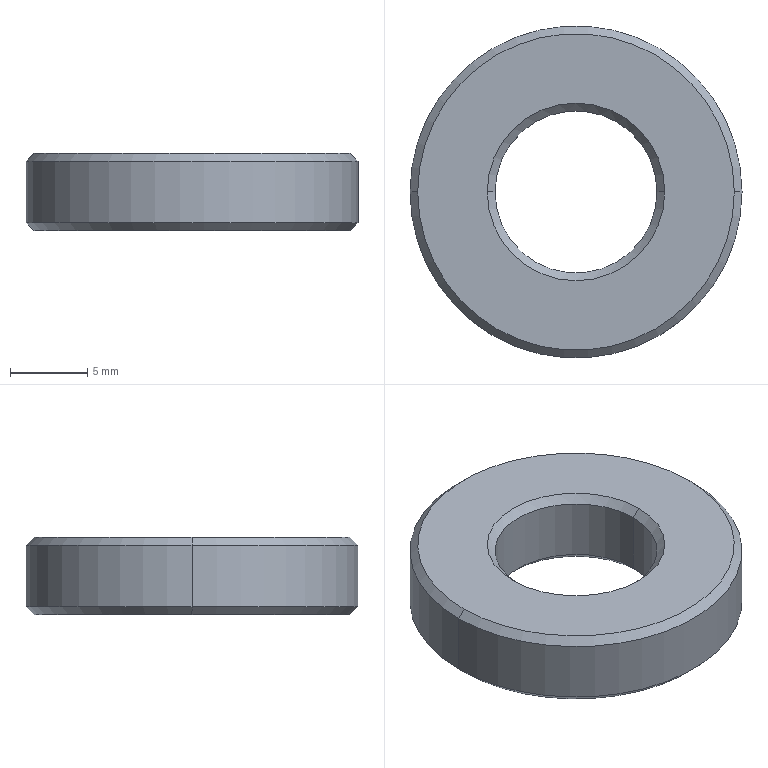Part | SolidWorks | features Chamfer 1, Extrusion 1 | 1 solid | 14 faces | box 21.5 x 21.5 x 5 mm | volume 1357 mm3 | cone 8 | cylinder 4 | plane 2 | commonest cylinder face diameters 10.5 x2 21.5 x2
STEP:
#1=CARTESIAN_POINT('',(10.25,0.,5.));
#2=VERTEX_POINT('',#1);
#3=CARTESIAN_POINT('',(-10.25,0.,5.));
#4=VERTEX_POINT('',#3);
#5=CARTESIAN_POINT('',(0.,0.,5.));
#6=DIRECTION('',(0.,0.,1.));
#7=DIRECTION('',(1.,0.,0.));
#8=AXIS2_PLACEMENT_3D('',#5,#6,#7);
#9=CIRCLE('',#8,10.25);
#10=EDGE_CURVE('',#2,#4,#9,.T.);
#11=ORIENTED_EDGE('',*,*,#10,.F.);
#12=CARTESIAN_POINT('',(10.75,0.,4.5));
#13=VERTEX_POINT('',#12);
#14=CARTESIAN_POINT('',(10.25,0.,5.));
#15=DIRECTION('',(0.7071,0.,-0.7071));
#16=VECTOR('',#15,1000.);
#17=LINE('',#14,#16);
#18=EDGE_CURVE('',#2,#13,#17,.T.);
#19=ORIENTED_EDGE('',*,*,#18,.T.);
#20=CARTESIAN_POINT('',(-10.75,0.,4.5));
#21=VERTEX_POINT('',#20);
#22=CARTESIAN_POINT('',(0.,0.,4.5));
#23=DIRECTION('',(0.,0.,-1.));
#24=DIRECTION('',(1.,0.,0.));
#25=AXIS2_PLACEMENT_3D('',#22,#23,#24);
#26=CIRCLE('',#25,10.75);
#27=EDGE_CURVE('',#21,#13,#26,.T.);
#28=ORIENTED_EDGE('',*,*,#27,.F.);
#29=CARTESIAN_POINT('',(-10.25,0.,5.));
#30=DIRECTION('',(-0.7071,0.,-0.7071));
#31=VECTOR('',#30,1000.);
#32=LINE('',#29,#31);
#33=EDGE_CURVE('',#4,#21,#32,.T.);
#34=ORIENTED_EDGE('',*,*,#33,.F.);
#35=EDGE_LOOP('',(#11,#19,#28,#34));
#36=FACE_OUTER_BOUND('',#35,.T.);
#37=CARTESIAN_POINT('',(0.,0.,5.));
#38=DIRECTION('',(0.,0.,-1.));
#39=DIRECTION('',(-1.,0.,0.));
#40=AXIS2_PLACEMENT_3D('',#37,#38,#39);
#41=CONICAL_SURFACE('',#40,10.25,0.7854);
#42=ADVANCED_FACE('',(#36),#41,.T.);
#43=CARTESIAN_POINT('',(-5.25,0.,4.5));
#44=VERTEX_POINT('',#43);
#45=CARTESIAN_POINT('',(5.25,0.,4.5));
#46=VERTEX_POINT('',#45);
#47=CARTESIAN_POINT('',(0.,0.,4.5));
#48=DIRECTION('',(0.,0.,1.));
#49=DIRECTION('',(1.,0.,0.));
#50=AXIS2_PLACEMENT_3D('',#47,#48,#49);
#51=CIRCLE('',#50,5.25);
#52=EDGE_CURVE('',#44,#46,#51,.T.);
#53=ORIENTED_EDGE('',*,*,#52,.F.);
#54=CARTESIAN_POINT('',(-5.75,0.,5.));
#55=VERTEX_POINT('',#54);
#56=CARTESIAN_POINT('',(-5.25,0.,4.5));
#57=DIRECTION('',(-0.7071,0.,0.7071));
#58=VECTOR('',#57,1000.);
#59=LINE('',#56,#58);
#60=EDGE_CURVE('',#44,#55,#59,.T.);
#61=ORIENTED_EDGE('',*,*,#60,.T.);
#62=CARTESIAN_POINT('',(5.75,0.,5.));
#63=VERTEX_POINT('',#62);
#64=CARTESIAN_POINT('',(0.,0.,5.));
#65=DIRECTION('',(0.,0.,-1.));
#66=DIRECTION('',(1.,0.,0.));
#67=AXIS2_PLACEMENT_3D('',#64,#65,#66);
#68=CIRCLE('',#67,5.75);
#69=EDGE_CURVE('',#63,#55,#68,.T.);
#70=ORIENTED_EDGE('',*,*,#69,.F.);
#71=CARTESIAN_POINT('',(5.25,0.,4.5));
#72=DIRECTION('',(0.7071,0.,0.7071));
#73=VECTOR('',#72,1000.);
#74=LINE('',#71,#73);
#75=EDGE_CURVE('',#46,#63,#74,.T.);
#76=ORIENTED_EDGE('',*,*,#75,.F.);
#77=EDGE_LOOP('',(#53,#61,#70,#76));
#78=FACE_OUTER_BOUND('',#77,.T.);
#79=CARTESIAN_POINT('',(0.,0.,4.5));
#80=DIRECTION('',(0.,0.,1.));
#81=DIRECTION('',(1.,0.,0.));
#82=AXIS2_PLACEMENT_3D('',#79,#80,#81);
#83=CONICAL_SURFACE('',#82,5.25,0.7854);
#84=ADVANCED_FACE('',(#78),#83,.F.);
#85=CARTESIAN_POINT('',(5.25,0.,0.5));
#86=VERTEX_POINT('',#85);
#87=CARTESIAN_POINT('',(-5.25,0.,0.5));
#88=VERTEX_POINT('',#87);
#89=CARTESIAN_POINT('',(0.,0.,0.5));
#90=DIRECTION('',(0.,0.,-1.));
#91=DIRECTION('',(1.,0.,0.));
#92=AXIS2_PLACEMENT_3D('',#89,#90,#91);
#93=CIRCLE('',#92,5.25);
#94=EDGE_CURVE('',#86,#88,#93,.T.);
#95=ORIENTED_EDGE('',*,*,#94,.F.);
#96=CARTESIAN_POINT('',(5.75,0.,0.));
#97=VERTEX_POINT('',#96);
#98=CARTESIAN_POINT('',(5.75,0.,0.));
#99=DIRECTION('',(0.7071,0.,-0.7071));
#100=VECTOR('',#99,1000.);
#101=LINE('',#98,#100);
#102=EDGE_CURVE('',#86,#97,#101,.T.);
#103=ORIENTED_EDGE('',*,*,#102,.T.);
#104=CARTESIAN_POINT('',(-5.75,0.,0.));
#105=VERTEX_POINT('',#104);
#106=CARTESIAN_POINT('',(0.,0.,0.));
#107=DIRECTION('',(0.,0.,1.));
#108=DIRECTION('',(1.,0.,0.));
#109=AXIS2_PLACEMENT_3D('',#106,#107,#108);
#110=CIRCLE('',#109,5.75);
#111=EDGE_CURVE('',#105,#97,#110,.T.);
#112=ORIENTED_EDGE('',*,*,#111,.F.);
#113=CARTESIAN_POINT('',(-5.75,0.,0.));
#114=DIRECTION('',(-0.7071,0.,-0.7071));
#115=VECTOR('',#114,1000.);
#116=LINE('',#113,#115);
#117=EDGE_CURVE('',#88,#105,#116,.T.);
#118=ORIENTED_EDGE('',*,*,#117,.F.);
#119=EDGE_LOOP('',(#95,#103,#112,#118));
#120=FACE_OUTER_BOUND('',#119,.T.);
#121=CARTESIAN_POINT('',(0.,0.,0.));
#122=DIRECTION('',(0.,0.,-1.));
#123=DIRECTION('',(-1.,0.,0.));
#124=AXIS2_PLACEMENT_3D('',#121,#122,#123);
#125=CONICAL_SURFACE('',#124,5.75,0.7854);
#126=ADVANCED_FACE('',(#120),#125,.F.);
#127=CARTESIAN_POINT('',(-10.25,0.,0.));
#128=VERTEX_POINT('',#127);
#129=CARTESIAN_POINT('',(10.25,0.,0.));
#130=VERTEX_POINT('',#129);
#131=CARTESIAN_POINT('',(0.,0.,0.));
#132=DIRECTION('',(0.,0.,-1.));
#133=DIRECTION('',(1.,0.,0.));
#134=AXIS2_PLACEMENT_3D('',#131,#132,#133);
#135=CIRCLE('',#134,10.25);
#136=EDGE_CURVE('',#128,#130,#135,.T.);
#137=ORIENTED_EDGE('',*,*,#136,.F.);
#138=CARTESIAN_POINT('',(-10.75,0.,0.5));
#139=VERTEX_POINT('',#138);
#140=CARTESIAN_POINT('',(-10.75,0.,0.5));
#141=DIRECTION('',(-0.7071,0.,0.7071));
#142=VECTOR('',#141,1000.);
#143=LINE('',#140,#142);
#144=EDGE_CURVE('',#128,#139,#143,.T.);
#145=ORIENTED_EDGE('',*,*,#144,.T.);
#146=CARTESIAN_POINT('',(10.75,0.,0.5));
#147=VERTEX_POINT('',#146);
#148=CARTESIAN_POINT('',(0.,0.,0.5));
#149=DIRECTION('',(0.,0.,1.));
#150=DIRECTION('',(1.,0.,0.));
#151=AXIS2_PLACEMENT_3D('',#148,#149,#150);
#152=CIRCLE('',#151,10.75);
#153=EDGE_CURVE('',#147,#139,#152,.T.);
#154=ORIENTED_EDGE('',*,*,#153,.F.);
#155=CARTESIAN_POINT('',(10.75,0.,0.5));
#156=DIRECTION('',(0.7071,0.,0.7071));
#157=VECTOR('',#156,1000.);
#158=LINE('',#155,#157);
#159=EDGE_CURVE('',#130,#147,#158,.T.);
#160=ORIENTED_EDGE('',*,*,#159,.F.);
#161=EDGE_LOOP('',(#137,#145,#154,#160));
#162=FACE_OUTER_BOUND('',#161,.T.);
#163=CARTESIAN_POINT('',(0.,0.,0.5));
#164=DIRECTION('',(0.,0.,1.));
#165=DIRECTION('',(1.,0.,0.));
#166=AXIS2_PLACEMENT_3D('',#163,#164,#165);
#167=CONICAL_SURFACE('',#166,10.75,0.7854);
#168=ADVANCED_FACE('',(#162),#167,.T.);
#169=ORIENTED_EDGE('',*,*,#52,.T.);
#170=CARTESIAN_POINT('',(5.25,0.,5.));
#171=DIRECTION('',(0.,0.,-1.));
#172=VECTOR('',#171,1000.);
#173=LINE('',#170,#172);
#174=EDGE_CURVE('',#46,#86,#173,.T.);
#175=ORIENTED_EDGE('',*,*,#174,.T.);
#176=ORIENTED_EDGE('',*,*,#94,.T.);
#177=CARTESIAN_POINT('',(-5.25,0.,5.));
#178=DIRECTION('',(0.,0.,-1.));
#179=VECTOR('',#178,1000.);
#180=LINE('',#177,#179);
#181=EDGE_CURVE('',#44,#88,#180,.T.);
#182=ORIENTED_EDGE('',*,*,#181,.F.);
#183=EDGE_LOOP('',(#169,#175,#176,#182));
#184=FACE_OUTER_BOUND('',#183,.T.);
#185=CARTESIAN_POINT('',(0.,0.,5.));
#186=DIRECTION('',(0.,0.,-1.));
#187=DIRECTION('',(-1.,0.,0.));
#188=AXIS2_PLACEMENT_3D('',#185,#186,#187);
#189=CYLINDRICAL_SURFACE('',#188,5.25);
#190=ADVANCED_FACE('',(#184),#189,.F.);
#191=ORIENTED_EDGE('',*,*,#27,.T.);
#192=CARTESIAN_POINT('',(10.75,0.,5.));
#193=DIRECTION('',(0.,0.,-1.));
#194=VECTOR('',#193,1000.);
#195=LINE('',#192,#194);
#196=EDGE_CURVE('',#13,#147,#195,.T.);
#197=ORIENTED_EDGE('',*,*,#196,.T.);
#198=ORIENTED_EDGE('',*,*,#153,.T.);
#199=CARTESIAN_POINT('',(-10.75,0.,5.));
#200=DIRECTION('',(0.,0.,-1.));
#201=VECTOR('',#200,1000.);
#202=LINE('',#199,#201);
#203=EDGE_CURVE('',#21,#139,#202,.T.);
#204=ORIENTED_EDGE('',*,*,#203,.F.);
#205=EDGE_LOOP('',(#191,#197,#198,#204));
#206=FACE_OUTER_BOUND('',#205,.T.);
#207=CARTESIAN_POINT('',(0.,0.,5.));
#208=DIRECTION('',(0.,0.,-1.));
#209=DIRECTION('',(-1.,0.,0.));
#210=AXIS2_PLACEMENT_3D('',#207,#208,#209);
#211=CYLINDRICAL_SURFACE('',#210,10.75);
#212=ADVANCED_FACE('',(#206),#211,.T.);
#213=ORIENTED_EDGE('',*,*,#69,.T.);
#214=CARTESIAN_POINT('',(0.,0.,5.));
#215=DIRECTION('',(0.,0.,-1.));
#216=DIRECTION('',(1.,0.,0.));
#217=AXIS2_PLACEMENT_3D('',#214,#215,#216);
#218=CIRCLE('',#217,5.75);
#219=EDGE_CURVE('',#55,#63,#218,.T.);
#220=ORIENTED_EDGE('',*,*,#219,.T.);
#221=EDGE_LOOP('',(#213,#220));
#222=FACE_BOUND('',#221,.T.);
#223=CARTESIAN_POINT('',(0.,0.,5.));
#224=DIRECTION('',(0.,0.,1.));
#225=DIRECTION('',(1.,0.,0.));
#226=AXIS2_PLACEMENT_3D('',#223,#224,#225);
#227=CIRCLE('',#226,10.25);
#228=EDGE_CURVE('',#4,#2,#227,.T.);
#229=ORIENTED_EDGE('',*,*,#228,.T.);
#230=ORIENTED_EDGE('',*,*,#10,.T.);
#231=EDGE_LOOP('',(#229,#230));
#232=FACE_OUTER_BOUND('',#231,.T.);
#233=CARTESIAN_POINT('',(0.,0.,5.));
#234=DIRECTION('',(0.,0.,1.));
#235=DIRECTION('',(1.,0.,0.));
#236=AXIS2_PLACEMENT_3D('',#233,#234,#235);
#237=PLANE('',#236);
#238=ADVANCED_FACE('',(#222,#232),#237,.T.);
#239=CARTESIAN_POINT('',(0.,0.,0.));
#240=DIRECTION('',(0.,0.,-1.));
#241=DIRECTION('',(1.,0.,0.));
#242=AXIS2_PLACEMENT_3D('',#239,#240,#241);
#243=CIRCLE('',#242,10.25);
#244=EDGE_CURVE('',#130,#128,#243,.T.);
#245=ORIENTED_EDGE('',*,*,#244,.T.);
#246=ORIENTED_EDGE('',*,*,#136,.T.);
#247=EDGE_LOOP('',(#245,#246));
#248=FACE_OUTER_BOUND('',#247,.T.);
#249=ORIENTED_EDGE('',*,*,#111,.T.);
#250=CARTESIAN_POINT('',(0.,0.,0.));
#251=DIRECTION('',(0.,0.,1.));
#252=DIRECTION('',(1.,0.,0.));
#253=AXIS2_PLACEMENT_3D('',#250,#251,#252);
#254=CIRCLE('',#253,5.75);
#255=EDGE_CURVE('',#97,#105,#254,.T.);
#256=ORIENTED_EDGE('',*,*,#255,.T.);
#257=EDGE_LOOP('',(#249,#256));
#258=FACE_BOUND('',#257,.T.);
#259=CARTESIAN_POINT('',(0.,0.,0.));
#260=DIRECTION('',(0.,0.,1.));
#261=DIRECTION('',(1.,0.,0.));
#262=AXIS2_PLACEMENT_3D('',#259,#260,#261);
#263=PLANE('',#262);
#264=ADVANCED_FACE('',(#248,#258),#263,.F.);
#265=ORIENTED_EDGE('',*,*,#196,.F.);
#266=CARTESIAN_POINT('',(0.,0.,4.5));
#267=DIRECTION('',(0.,0.,-1.));
#268=DIRECTION('',(1.,0.,0.));
#269=AXIS2_PLACEMENT_3D('',#266,#267,#268);
#270=CIRCLE('',#269,10.75);
#271=EDGE_CURVE('',#13,#21,#270,.T.);
#272=ORIENTED_EDGE('',*,*,#271,.T.);
#273=ORIENTED_EDGE('',*,*,#203,.T.);
#274=CARTESIAN_POINT('',(0.,0.,0.5));
#275=DIRECTION('',(0.,0.,1.));
#276=DIRECTION('',(1.,0.,0.));
#277=AXIS2_PLACEMENT_3D('',#274,#275,#276);
#278=CIRCLE('',#277,10.75);
#279=EDGE_CURVE('',#139,#147,#278,.T.);
#280=ORIENTED_EDGE('',*,*,#279,.T.);
#281=EDGE_LOOP('',(#265,#272,#273,#280));
#282=FACE_OUTER_BOUND('',#281,.T.);
#283=CARTESIAN_POINT('',(0.,0.,5.));
#284=DIRECTION('',(0.,0.,-1.));
#285=DIRECTION('',(-1.,0.,0.));
#286=AXIS2_PLACEMENT_3D('',#283,#284,#285);
#287=CYLINDRICAL_SURFACE('',#286,10.75);
#288=ADVANCED_FACE('',(#282),#287,.T.);
#289=ORIENTED_EDGE('',*,*,#174,.F.);
#290=CARTESIAN_POINT('',(0.,0.,4.5));
#291=DIRECTION('',(0.,0.,1.));
#292=DIRECTION('',(1.,0.,0.));
#293=AXIS2_PLACEMENT_3D('',#290,#291,#292);
#294=CIRCLE('',#293,5.25);
#295=EDGE_CURVE('',#46,#44,#294,.T.);
#296=ORIENTED_EDGE('',*,*,#295,.T.);
#297=ORIENTED_EDGE('',*,*,#181,.T.);
#298=CARTESIAN_POINT('',(0.,0.,0.5));
#299=DIRECTION('',(0.,0.,-1.));
#300=DIRECTION('',(1.,0.,0.));
#301=AXIS2_PLACEMENT_3D('',#298,#299,#300);
#302=CIRCLE('',#301,5.25);
#303=EDGE_CURVE('',#88,#86,#302,.T.);
#304=ORIENTED_EDGE('',*,*,#303,.T.);
#305=EDGE_LOOP('',(#289,#296,#297,#304));
#306=FACE_OUTER_BOUND('',#305,.T.);
#307=CARTESIAN_POINT('',(0.,0.,5.));
#308=DIRECTION('',(0.,0.,-1.));
#309=DIRECTION('',(-1.,0.,0.));
#310=AXIS2_PLACEMENT_3D('',#307,#308,#309);
#311=CYLINDRICAL_SURFACE('',#310,5.25);
#312=ADVANCED_FACE('',(#306),#311,.F.);
#313=ORIENTED_EDGE('',*,*,#144,.F.);
#314=ORIENTED_EDGE('',*,*,#244,.F.);
#315=ORIENTED_EDGE('',*,*,#159,.T.);
#316=ORIENTED_EDGE('',*,*,#279,.F.);
#317=EDGE_LOOP('',(#313,#314,#315,#316));
#318=FACE_OUTER_BOUND('',#317,.T.);
#319=CARTESIAN_POINT('',(0.,0.,0.5));
#320=DIRECTION('',(0.,0.,1.));
#321=DIRECTION('',(1.,0.,0.));
#322=AXIS2_PLACEMENT_3D('',#319,#320,#321);
#323=CONICAL_SURFACE('',#322,10.75,0.7854);
#324=ADVANCED_FACE('',(#318),#323,.T.);
#325=ORIENTED_EDGE('',*,*,#102,.F.);
#326=ORIENTED_EDGE('',*,*,#303,.F.);
#327=ORIENTED_EDGE('',*,*,#117,.T.);
#328=ORIENTED_EDGE('',*,*,#255,.F.);
#329=EDGE_LOOP('',(#325,#326,#327,#328));
#330=FACE_OUTER_BOUND('',#329,.T.);
#331=CARTESIAN_POINT('',(0.,0.,0.));
#332=DIRECTION('',(0.,0.,-1.));
#333=DIRECTION('',(-1.,0.,0.));
#334=AXIS2_PLACEMENT_3D('',#331,#332,#333);
#335=CONICAL_SURFACE('',#334,5.75,0.7854);
#336=ADVANCED_FACE('',(#330),#335,.F.);
#337=ORIENTED_EDGE('',*,*,#60,.F.);
#338=ORIENTED_EDGE('',*,*,#295,.F.);
#339=ORIENTED_EDGE('',*,*,#75,.T.);
#340=ORIENTED_EDGE('',*,*,#219,.F.);
#341=EDGE_LOOP('',(#337,#338,#339,#340));
#342=FACE_OUTER_BOUND('',#341,.T.);
#343=CARTESIAN_POINT('',(0.,0.,4.5));
#344=DIRECTION('',(0.,0.,1.));
#345=DIRECTION('',(1.,0.,0.));
#346=AXIS2_PLACEMENT_3D('',#343,#344,#345);
#347=CONICAL_SURFACE('',#346,5.25,0.7854);
#348=ADVANCED_FACE('',(#342),#347,.F.);
#349=ORIENTED_EDGE('',*,*,#18,.F.);
#350=ORIENTED_EDGE('',*,*,#228,.F.);
#351=ORIENTED_EDGE('',*,*,#33,.T.);
#352=ORIENTED_EDGE('',*,*,#271,.F.);
#353=EDGE_LOOP('',(#349,#350,#351,#352));
#354=FACE_OUTER_BOUND('',#353,.T.);
#355=CARTESIAN_POINT('',(0.,0.,5.));
#356=DIRECTION('',(0.,0.,-1.));
#357=DIRECTION('',(-1.,0.,0.));
#358=AXIS2_PLACEMENT_3D('',#355,#356,#357);
#359=CONICAL_SURFACE('',#358,10.25,0.7854);
#360=ADVANCED_FACE('',(#354),#359,.T.);
#361=CLOSED_SHELL('',(#42,#84,#126,#168,#190,#212,#238,#264,#288,#312,#324,#336,#348,#360));
#362=MANIFOLD_SOLID_BREP('',#361);
#363=CARTESIAN_POINT('',(0.,0.,0.));
#364=DIRECTION('',(0.,0.,1.));
#365=DIRECTION('',(1.,0.,0.));
#366=AXIS2_PLACEMENT_3D('',#363,#364,#365);
#367=(LENGTH_UNIT()NAMED_UNIT(*)SI_UNIT(.MILLI.,.METRE.));
#368=UNCERTAINTY_MEASURE_WITH_UNIT(LENGTH_MEASURE(0.00001),#367,'','');
#369=(NAMED_UNIT(*)PLANE_ANGLE_UNIT()SI_UNIT($,.RADIAN.));
#370=(NAMED_UNIT(*)SI_UNIT($,.STERADIAN.)SOLID_ANGLE_UNIT());
#371=(GEOMETRIC_REPRESENTATION_CONTEXT(3)GLOBAL_UNCERTAINTY_ASSIGNED_CONTEXT((#368))GLOBAL_UNIT_ASSIGNED_CONTEXT((#367,#369,#370))REPRESENTATION_CONTEXT('',''));
#372=ADVANCED_BREP_SHAPE_REPRESENTATION('',(#362,#366),#371);